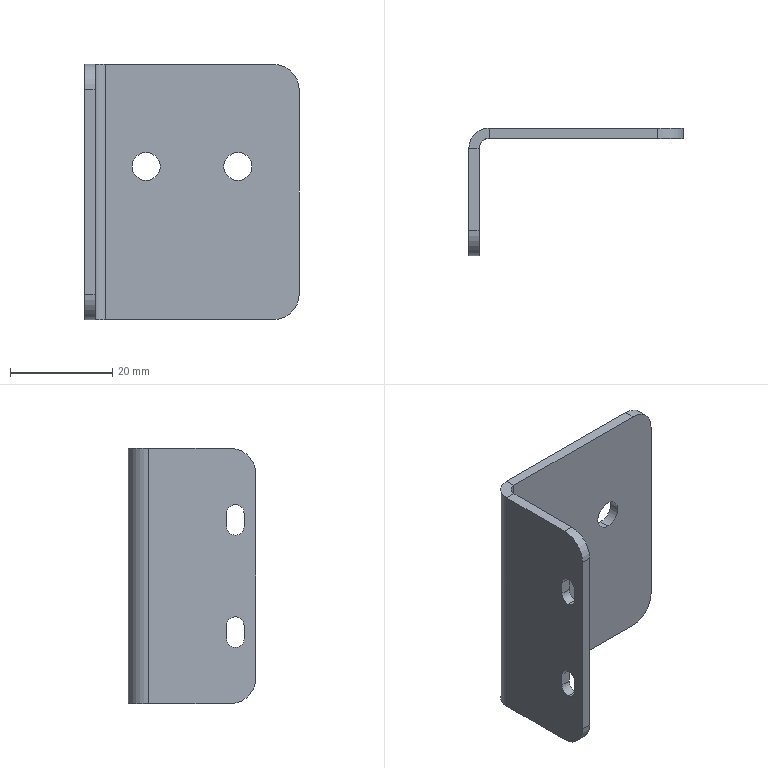Part | SolidWorks | features HoleWzd 3, EdgeFlange 2, Chamfer 1, Fillet 1, FlatPattern 1, MirrorPattern 1, SMBaseFlange 1, SheetMetal 1 | 1 solid | 32 faces | box 42 x 25 x 50 mm | volume 6162 mm3 | cylinder 16 | plane 16 | commonest cylinder face diameters 3.4 x6 5.5 x4 10 x4 4 x1 8 x1
STEP:
#1=CARTESIAN_POINT('',(28.,13.5,7.75));
#2=VERTEX_POINT('',#1);
#3=CARTESIAN_POINT('',(28.,13.5,2.25));
#4=VERTEX_POINT('',#3);
#5=CARTESIAN_POINT('',(28.,13.5,5.));
#6=DIRECTION('',(0.,-1.,0.));
#7=DIRECTION('',(0.,0.,-1.));
#8=AXIS2_PLACEMENT_3D('',#5,#6,#7);
#9=CIRCLE('',#8,2.75);
#10=EDGE_CURVE('',#2,#4,#9,.T.);
#11=ORIENTED_EDGE('',*,*,#10,.F.);
#12=CARTESIAN_POINT('',(28.,11.5,7.75));
#13=VERTEX_POINT('',#12);
#14=CARTESIAN_POINT('',(28.,11.5,7.75));
#15=DIRECTION('',(0.,-1.,0.));
#16=VECTOR('',#15,1000.);
#17=LINE('',#14,#16);
#18=EDGE_CURVE('',#2,#13,#17,.T.);
#19=ORIENTED_EDGE('',*,*,#18,.T.);
#20=CARTESIAN_POINT('',(28.,11.5,2.25));
#21=VERTEX_POINT('',#20);
#22=CARTESIAN_POINT('',(28.,11.5,5.));
#23=DIRECTION('',(0.,-1.,0.));
#24=DIRECTION('',(0.,0.,-1.));
#25=AXIS2_PLACEMENT_3D('',#22,#23,#24);
#26=CIRCLE('',#25,2.75);
#27=EDGE_CURVE('',#13,#21,#26,.T.);
#28=ORIENTED_EDGE('',*,*,#27,.T.);
#29=CARTESIAN_POINT('',(28.,11.5,2.25));
#30=DIRECTION('',(0.,-1.,0.));
#31=VECTOR('',#30,1000.);
#32=LINE('',#29,#31);
#33=EDGE_CURVE('',#4,#21,#32,.T.);
#34=ORIENTED_EDGE('',*,*,#33,.F.);
#35=EDGE_LOOP('',(#11,#19,#28,#34));
#36=FACE_OUTER_BOUND('',#35,.T.);
#37=CARTESIAN_POINT('',(28.,11.5,5.));
#38=DIRECTION('',(0.,-1.,0.));
#39=DIRECTION('',(0.,0.,-1.));
#40=AXIS2_PLACEMENT_3D('',#37,#38,#39);
#41=CYLINDRICAL_SURFACE('',#40,2.75);
#42=ADVANCED_FACE('',(#36),#41,.F.);
#43=CARTESIAN_POINT('',(10.,13.5,7.75));
#44=VERTEX_POINT('',#43);
#45=CARTESIAN_POINT('',(10.,13.5,2.25));
#46=VERTEX_POINT('',#45);
#47=CARTESIAN_POINT('',(10.,13.5,5.));
#48=DIRECTION('',(0.,-1.,0.));
#49=DIRECTION('',(0.,0.,-1.));
#50=AXIS2_PLACEMENT_3D('',#47,#48,#49);
#51=CIRCLE('',#50,2.75);
#52=EDGE_CURVE('',#44,#46,#51,.T.);
#53=ORIENTED_EDGE('',*,*,#52,.F.);
#54=CARTESIAN_POINT('',(10.,11.5,7.75));
#55=VERTEX_POINT('',#54);
#56=CARTESIAN_POINT('',(10.,11.5,7.75));
#57=DIRECTION('',(0.,-1.,0.));
#58=VECTOR('',#57,1000.);
#59=LINE('',#56,#58);
#60=EDGE_CURVE('',#44,#55,#59,.T.);
#61=ORIENTED_EDGE('',*,*,#60,.T.);
#62=CARTESIAN_POINT('',(10.,11.5,2.25));
#63=VERTEX_POINT('',#62);
#64=CARTESIAN_POINT('',(10.,11.5,5.));
#65=DIRECTION('',(0.,-1.,0.));
#66=DIRECTION('',(0.,0.,-1.));
#67=AXIS2_PLACEMENT_3D('',#64,#65,#66);
#68=CIRCLE('',#67,2.75);
#69=EDGE_CURVE('',#55,#63,#68,.T.);
#70=ORIENTED_EDGE('',*,*,#69,.T.);
#71=CARTESIAN_POINT('',(10.,11.5,2.25));
#72=DIRECTION('',(0.,-1.,0.));
#73=VECTOR('',#72,1000.);
#74=LINE('',#71,#73);
#75=EDGE_CURVE('',#46,#63,#74,.T.);
#76=ORIENTED_EDGE('',*,*,#75,.F.);
#77=EDGE_LOOP('',(#53,#61,#70,#76));
#78=FACE_OUTER_BOUND('',#77,.T.);
#79=CARTESIAN_POINT('',(10.,11.5,5.));
#80=DIRECTION('',(0.,-1.,0.));
#81=DIRECTION('',(0.,0.,-1.));
#82=AXIS2_PLACEMENT_3D('',#79,#80,#81);
#83=CYLINDRICAL_SURFACE('',#82,2.75);
#84=ADVANCED_FACE('',(#78),#83,.F.);
#85=CARTESIAN_POINT('',(-2.,-7.5,-14.));
#86=VERTEX_POINT('',#85);
#87=CARTESIAN_POINT('',(-2.,-5.8,-12.3));
#88=VERTEX_POINT('',#87);
#89=CARTESIAN_POINT('',(-2.,-7.5,-12.3));
#90=DIRECTION('',(1.,0.,0.));
#91=DIRECTION('',(0.,0.,-1.));
#92=AXIS2_PLACEMENT_3D('',#89,#90,#91);
#93=CIRCLE('',#92,1.7);
#94=EDGE_CURVE('',#86,#88,#93,.T.);
#95=ORIENTED_EDGE('',*,*,#94,.F.);
#96=CARTESIAN_POINT('',(0.,-7.5,-14.));
#97=VERTEX_POINT('',#96);
#98=CARTESIAN_POINT('',(0.,-7.5,-14.));
#99=DIRECTION('',(1.,0.,0.));
#100=VECTOR('',#99,1000.);
#101=LINE('',#98,#100);
#102=EDGE_CURVE('',#86,#97,#101,.T.);
#103=ORIENTED_EDGE('',*,*,#102,.T.);
#104=CARTESIAN_POINT('',(0.,-5.8,-12.3));
#105=VERTEX_POINT('',#104);
#106=CARTESIAN_POINT('',(0.,-7.5,-12.3));
#107=DIRECTION('',(1.,0.,0.));
#108=DIRECTION('',(0.,0.,-1.));
#109=AXIS2_PLACEMENT_3D('',#106,#107,#108);
#110=CIRCLE('',#109,1.7);
#111=EDGE_CURVE('',#97,#105,#110,.T.);
#112=ORIENTED_EDGE('',*,*,#111,.T.);
#113=CARTESIAN_POINT('',(-2.,-5.8,-12.3));
#114=DIRECTION('',(-1.,0.,0.));
#115=VECTOR('',#114,1000.);
#116=LINE('',#113,#115);
#117=EDGE_CURVE('',#105,#88,#116,.T.);
#118=ORIENTED_EDGE('',*,*,#117,.T.);
#119=EDGE_LOOP('',(#95,#103,#112,#118));
#120=FACE_OUTER_BOUND('',#119,.T.);
#121=CARTESIAN_POINT('',(0.,-7.5,-12.3));
#122=DIRECTION('',(1.,0.,0.));
#123=DIRECTION('',(0.,0.,-1.));
#124=AXIS2_PLACEMENT_3D('',#121,#122,#123);
#125=CYLINDRICAL_SURFACE('',#124,1.7);
#126=ADVANCED_FACE('',(#120),#125,.F.);
#127=CARTESIAN_POINT('',(-2.,-7.5,8.));
#128=VERTEX_POINT('',#127);
#129=CARTESIAN_POINT('',(-2.,-5.8,9.7));
#130=VERTEX_POINT('',#129);
#131=CARTESIAN_POINT('',(-2.,-7.5,9.7));
#132=DIRECTION('',(1.,0.,0.));
#133=DIRECTION('',(0.,0.,-1.));
#134=AXIS2_PLACEMENT_3D('',#131,#132,#133);
#135=CIRCLE('',#134,1.7);
#136=EDGE_CURVE('',#128,#130,#135,.T.);
#137=ORIENTED_EDGE('',*,*,#136,.F.);
#138=CARTESIAN_POINT('',(0.,-7.5,8.));
#139=VERTEX_POINT('',#138);
#140=CARTESIAN_POINT('',(0.,-7.5,8.));
#141=DIRECTION('',(1.,0.,0.));
#142=VECTOR('',#141,1000.);
#143=LINE('',#140,#142);
#144=EDGE_CURVE('',#128,#139,#143,.T.);
#145=ORIENTED_EDGE('',*,*,#144,.T.);
#146=CARTESIAN_POINT('',(0.,-5.8,9.7));
#147=VERTEX_POINT('',#146);
#148=CARTESIAN_POINT('',(0.,-7.5,9.7));
#149=DIRECTION('',(1.,0.,0.));
#150=DIRECTION('',(0.,0.,-1.));
#151=AXIS2_PLACEMENT_3D('',#148,#149,#150);
#152=CIRCLE('',#151,1.7);
#153=EDGE_CURVE('',#139,#147,#152,.T.);
#154=ORIENTED_EDGE('',*,*,#153,.T.);
#155=CARTESIAN_POINT('',(-2.,-5.8,9.7));
#156=DIRECTION('',(-1.,0.,0.));
#157=VECTOR('',#156,1000.);
#158=LINE('',#155,#157);
#159=EDGE_CURVE('',#147,#130,#158,.T.);
#160=ORIENTED_EDGE('',*,*,#159,.T.);
#161=EDGE_LOOP('',(#137,#145,#154,#160));
#162=FACE_OUTER_BOUND('',#161,.T.);
#163=CARTESIAN_POINT('',(0.,-7.5,9.7));
#164=DIRECTION('',(1.,0.,0.));
#165=DIRECTION('',(0.,0.,-1.));
#166=AXIS2_PLACEMENT_3D('',#163,#164,#165);
#167=CYLINDRICAL_SURFACE('',#166,1.7);
#168=ADVANCED_FACE('',(#162),#167,.F.);
#169=CARTESIAN_POINT('',(-2.,9.5,25.));
#170=VERTEX_POINT('',#169);
#171=CARTESIAN_POINT('',(-2.,-6.5,25.));
#172=VERTEX_POINT('',#171);
#173=CARTESIAN_POINT('',(-2.,11.5,25.));
#174=DIRECTION('',(0.,-1.,0.));
#175=VECTOR('',#174,1000.);
#176=LINE('',#173,#175);
#177=EDGE_CURVE('',#170,#172,#176,.T.);
#178=ORIENTED_EDGE('',*,*,#177,.T.);
#179=CARTESIAN_POINT('',(0.,-6.5,25.));
#180=VERTEX_POINT('',#179);
#181=CARTESIAN_POINT('',(-2.,-6.5,25.));
#182=DIRECTION('',(1.,0.,0.));
#183=VECTOR('',#182,1000.);
#184=LINE('',#181,#183);
#185=EDGE_CURVE('',#172,#180,#184,.T.);
#186=ORIENTED_EDGE('',*,*,#185,.T.);
#187=CARTESIAN_POINT('',(0.,9.5,25.));
#188=VERTEX_POINT('',#187);
#189=CARTESIAN_POINT('',(0.,11.5,25.));
#190=DIRECTION('',(0.,-1.,0.));
#191=VECTOR('',#190,1000.);
#192=LINE('',#189,#191);
#193=EDGE_CURVE('',#188,#180,#192,.T.);
#194=ORIENTED_EDGE('',*,*,#193,.F.);
#195=CARTESIAN_POINT('',(0.,9.5,25.));
#196=DIRECTION('',(-1.,0.,0.));
#197=VECTOR('',#196,1000.);
#198=LINE('',#195,#197);
#199=EDGE_CURVE('',#188,#170,#198,.T.);
#200=ORIENTED_EDGE('',*,*,#199,.T.);
#201=EDGE_LOOP('',(#178,#186,#194,#200));
#202=FACE_OUTER_BOUND('',#201,.T.);
#203=CARTESIAN_POINT('',(-2.,11.5,25.));
#204=DIRECTION('',(0.,0.,1.));
#205=DIRECTION('',(0.,-1.,0.));
#206=AXIS2_PLACEMENT_3D('',#203,#204,#205);
#207=PLANE('',#206);
#208=ADVANCED_FACE('',(#202),#207,.T.);
#209=CARTESIAN_POINT('',(-2.,-5.8,12.3));
#210=VERTEX_POINT('',#209);
#211=CARTESIAN_POINT('',(-2.,-9.2,12.3));
#212=VERTEX_POINT('',#211);
#213=CARTESIAN_POINT('',(-2.,-7.5,12.3));
#214=DIRECTION('',(1.,0.,0.));
#215=DIRECTION('',(0.,0.,-1.));
#216=AXIS2_PLACEMENT_3D('',#213,#214,#215);
#217=CIRCLE('',#216,1.7);
#218=EDGE_CURVE('',#210,#212,#217,.T.);
#219=ORIENTED_EDGE('',*,*,#218,.T.);
#220=CARTESIAN_POINT('',(-2.,-9.2,9.7));
#221=VERTEX_POINT('',#220);
#222=CARTESIAN_POINT('',(-2.,-9.2,12.3));
#223=DIRECTION('',(0.,0.,-1.));
#224=VECTOR('',#223,1000.);
#225=LINE('',#222,#224);
#226=EDGE_CURVE('',#212,#221,#225,.T.);
#227=ORIENTED_EDGE('',*,*,#226,.T.);
#228=CARTESIAN_POINT('',(-2.,-7.5,9.7));
#229=DIRECTION('',(1.,0.,0.));
#230=DIRECTION('',(0.,0.,-1.));
#231=AXIS2_PLACEMENT_3D('',#228,#229,#230);
#232=CIRCLE('',#231,1.7);
#233=EDGE_CURVE('',#221,#128,#232,.T.);
#234=ORIENTED_EDGE('',*,*,#233,.T.);
#235=ORIENTED_EDGE('',*,*,#136,.T.);
#236=CARTESIAN_POINT('',(-2.,-5.8,12.3));
#237=DIRECTION('',(0.,0.,-1.));
#238=VECTOR('',#237,1000.);
#239=LINE('',#236,#238);
#240=EDGE_CURVE('',#210,#130,#239,.T.);
#241=ORIENTED_EDGE('',*,*,#240,.F.);
#242=EDGE_LOOP('',(#219,#227,#234,#235,#241));
#243=FACE_BOUND('',#242,.T.);
#244=CARTESIAN_POINT('',(-2.,-5.8,-9.7));
#245=VERTEX_POINT('',#244);
#246=CARTESIAN_POINT('',(-2.,-5.8,-9.7));
#247=DIRECTION('',(0.,0.,-1.));
#248=VECTOR('',#247,1000.);
#249=LINE('',#246,#248);
#250=EDGE_CURVE('',#245,#88,#249,.T.);
#251=ORIENTED_EDGE('',*,*,#250,.F.);
#252=CARTESIAN_POINT('',(-2.,-9.2,-9.7));
#253=VERTEX_POINT('',#252);
#254=CARTESIAN_POINT('',(-2.,-7.5,-9.7));
#255=DIRECTION('',(1.,0.,0.));
#256=DIRECTION('',(0.,0.,-1.));
#257=AXIS2_PLACEMENT_3D('',#254,#255,#256);
#258=CIRCLE('',#257,1.7);
#259=EDGE_CURVE('',#245,#253,#258,.T.);
#260=ORIENTED_EDGE('',*,*,#259,.T.);
#261=CARTESIAN_POINT('',(-2.,-9.2,-12.3));
#262=VERTEX_POINT('',#261);
#263=CARTESIAN_POINT('',(-2.,-9.2,-9.7));
#264=DIRECTION('',(0.,0.,-1.));
#265=VECTOR('',#264,1000.);
#266=LINE('',#263,#265);
#267=EDGE_CURVE('',#253,#262,#266,.T.);
#268=ORIENTED_EDGE('',*,*,#267,.T.);
#269=CARTESIAN_POINT('',(-2.,-7.5,-12.3));
#270=DIRECTION('',(1.,0.,0.));
#271=DIRECTION('',(0.,0.,-1.));
#272=AXIS2_PLACEMENT_3D('',#269,#270,#271);
#273=CIRCLE('',#272,1.7);
#274=EDGE_CURVE('',#262,#86,#273,.T.);
#275=ORIENTED_EDGE('',*,*,#274,.T.);
#276=ORIENTED_EDGE('',*,*,#94,.T.);
#277=EDGE_LOOP('',(#251,#260,#268,#275,#276));
#278=FACE_BOUND('',#277,.T.);
#279=CARTESIAN_POINT('',(-2.,-11.5,20.));
#280=VERTEX_POINT('',#279);
#281=CARTESIAN_POINT('',(-2.,-11.5,-20.));
#282=VERTEX_POINT('',#281);
#283=CARTESIAN_POINT('',(-2.,-11.5,25.));
#284=DIRECTION('',(0.,0.,-1.));
#285=VECTOR('',#284,1000.);
#286=LINE('',#283,#285);
#287=EDGE_CURVE('',#280,#282,#286,.T.);
#288=ORIENTED_EDGE('',*,*,#287,.F.);
#289=CARTESIAN_POINT('',(-2.,-6.5,20.));
#290=DIRECTION('',(-1.,0.,0.));
#291=DIRECTION('',(0.,0.,-1.));
#292=AXIS2_PLACEMENT_3D('',#289,#290,#291);
#293=CIRCLE('',#292,5.);
#294=EDGE_CURVE('',#280,#172,#293,.T.);
#295=ORIENTED_EDGE('',*,*,#294,.T.);
#296=ORIENTED_EDGE('',*,*,#177,.F.);
#297=CARTESIAN_POINT('',(-2.,9.5,-25.));
#298=VERTEX_POINT('',#297);
#299=CARTESIAN_POINT('',(-2.,9.5,25.));
#300=DIRECTION('',(0.,0.,-1.));
#301=VECTOR('',#300,1000.);
#302=LINE('',#299,#301);
#303=EDGE_CURVE('',#170,#298,#302,.T.);
#304=ORIENTED_EDGE('',*,*,#303,.T.);
#305=CARTESIAN_POINT('',(-2.,-6.5,-25.));
#306=VERTEX_POINT('',#305);
#307=CARTESIAN_POINT('',(-2.,11.5,-25.));
#308=DIRECTION('',(0.,1.,0.));
#309=VECTOR('',#308,1000.);
#310=LINE('',#307,#309);
#311=EDGE_CURVE('',#306,#298,#310,.T.);
#312=ORIENTED_EDGE('',*,*,#311,.F.);
#313=CARTESIAN_POINT('',(-2.,-6.5,-20.));
#314=DIRECTION('',(-1.,0.,0.));
#315=DIRECTION('',(0.,0.,-1.));
#316=AXIS2_PLACEMENT_3D('',#313,#314,#315);
#317=CIRCLE('',#316,5.);
#318=EDGE_CURVE('',#306,#282,#317,.T.);
#319=ORIENTED_EDGE('',*,*,#318,.T.);
#320=EDGE_LOOP('',(#288,#295,#296,#304,#312,#319));
#321=FACE_OUTER_BOUND('',#320,.T.);
#322=CARTESIAN_POINT('',(-2.,0.,0.));
#323=DIRECTION('',(1.,0.,0.));
#324=DIRECTION('',(0.,0.,-1.));
#325=AXIS2_PLACEMENT_3D('',#322,#323,#324);
#326=PLANE('',#325);
#327=ADVANCED_FACE('',(#243,#278,#321),#326,.F.);
#328=CARTESIAN_POINT('',(0.,-9.2,-12.3));
#329=VERTEX_POINT('',#328);
#330=CARTESIAN_POINT('',(0.,-7.5,-12.3));
#331=DIRECTION('',(1.,0.,0.));
#332=DIRECTION('',(0.,0.,-1.));
#333=AXIS2_PLACEMENT_3D('',#330,#331,#332);
#334=CIRCLE('',#333,1.7);
#335=EDGE_CURVE('',#329,#97,#334,.T.);
#336=ORIENTED_EDGE('',*,*,#335,.F.);
#337=CARTESIAN_POINT('',(0.,-9.2,-9.7));
#338=VERTEX_POINT('',#337);
#339=CARTESIAN_POINT('',(0.,-9.2,-9.7));
#340=DIRECTION('',(0.,0.,-1.));
#341=VECTOR('',#340,1000.);
#342=LINE('',#339,#341);
#343=EDGE_CURVE('',#338,#329,#342,.T.);
#344=ORIENTED_EDGE('',*,*,#343,.F.);
#345=CARTESIAN_POINT('',(0.,-5.8,-9.7));
#346=VERTEX_POINT('',#345);
#347=CARTESIAN_POINT('',(0.,-7.5,-9.7));
#348=DIRECTION('',(1.,0.,0.));
#349=DIRECTION('',(0.,0.,-1.));
#350=AXIS2_PLACEMENT_3D('',#347,#348,#349);
#351=CIRCLE('',#350,1.7);
#352=EDGE_CURVE('',#346,#338,#351,.T.);
#353=ORIENTED_EDGE('',*,*,#352,.F.);
#354=CARTESIAN_POINT('',(0.,-5.8,-9.7));
#355=DIRECTION('',(0.,0.,-1.));
#356=VECTOR('',#355,1000.);
#357=LINE('',#354,#356);
#358=EDGE_CURVE('',#346,#105,#357,.T.);
#359=ORIENTED_EDGE('',*,*,#358,.T.);
#360=ORIENTED_EDGE('',*,*,#111,.F.);
#361=EDGE_LOOP('',(#336,#344,#353,#359,#360));
#362=FACE_BOUND('',#361,.T.);
#363=CARTESIAN_POINT('',(0.,-9.2,12.3));
#364=VERTEX_POINT('',#363);
#365=CARTESIAN_POINT('',(0.,-9.2,9.7));
#366=VERTEX_POINT('',#365);
#367=CARTESIAN_POINT('',(0.,-9.2,12.3));
#368=DIRECTION('',(0.,0.,-1.));
#369=VECTOR('',#368,1000.);
#370=LINE('',#367,#369);
#371=EDGE_CURVE('',#364,#366,#370,.T.);
#372=ORIENTED_EDGE('',*,*,#371,.F.);
#373=CARTESIAN_POINT('',(0.,-5.8,12.3));
#374=VERTEX_POINT('',#373);
#375=CARTESIAN_POINT('',(0.,-7.5,12.3));
#376=DIRECTION('',(1.,0.,0.));
#377=DIRECTION('',(0.,0.,-1.));
#378=AXIS2_PLACEMENT_3D('',#375,#376,#377);
#379=CIRCLE('',#378,1.7);
#380=EDGE_CURVE('',#374,#364,#379,.T.);
#381=ORIENTED_EDGE('',*,*,#380,.F.);
#382=CARTESIAN_POINT('',(0.,-5.8,12.3));
#383=DIRECTION('',(0.,0.,-1.));
#384=VECTOR('',#383,1000.);
#385=LINE('',#382,#384);
#386=EDGE_CURVE('',#374,#147,#385,.T.);
#387=ORIENTED_EDGE('',*,*,#386,.T.);
#388=ORIENTED_EDGE('',*,*,#153,.F.);
#389=CARTESIAN_POINT('',(0.,-7.5,9.7));
#390=DIRECTION('',(1.,0.,0.));
#391=DIRECTION('',(0.,0.,-1.));
#392=AXIS2_PLACEMENT_3D('',#389,#390,#391);
#393=CIRCLE('',#392,1.7);
#394=EDGE_CURVE('',#366,#139,#393,.T.);
#395=ORIENTED_EDGE('',*,*,#394,.F.);
#396=EDGE_LOOP('',(#372,#381,#387,#388,#395));
#397=FACE_BOUND('',#396,.T.);
#398=ORIENTED_EDGE('',*,*,#193,.T.);
#399=CARTESIAN_POINT('',(0.,-11.5,20.));
#400=VERTEX_POINT('',#399);
#401=CARTESIAN_POINT('',(0.,-6.5,20.));
#402=DIRECTION('',(1.,0.,0.));
#403=DIRECTION('',(0.,0.,-1.));
#404=AXIS2_PLACEMENT_3D('',#401,#402,#403);
#405=CIRCLE('',#404,5.);
#406=EDGE_CURVE('',#180,#400,#405,.T.);
#407=ORIENTED_EDGE('',*,*,#406,.T.);
#408=CARTESIAN_POINT('',(0.,-11.5,-20.));
#409=VERTEX_POINT('',#408);
#410=CARTESIAN_POINT('',(0.,-11.5,25.));
#411=DIRECTION('',(0.,0.,-1.));
#412=VECTOR('',#411,1000.);
#413=LINE('',#410,#412);
#414=EDGE_CURVE('',#400,#409,#413,.T.);
#415=ORIENTED_EDGE('',*,*,#414,.T.);
#416=CARTESIAN_POINT('',(0.,-6.5,-25.));
#417=VERTEX_POINT('',#416);
#418=CARTESIAN_POINT('',(0.,-6.5,-20.));
#419=DIRECTION('',(1.,0.,0.));
#420=DIRECTION('',(0.,0.,-1.));
#421=AXIS2_PLACEMENT_3D('',#418,#419,#420);
#422=CIRCLE('',#421,5.);
#423=EDGE_CURVE('',#409,#417,#422,.T.);
#424=ORIENTED_EDGE('',*,*,#423,.T.);
#425=CARTESIAN_POINT('',(0.,9.5,-25.));
#426=VERTEX_POINT('',#425);
#427=CARTESIAN_POINT('',(0.,11.5,-25.));
#428=DIRECTION('',(0.,1.,0.));
#429=VECTOR('',#428,1000.);
#430=LINE('',#427,#429);
#431=EDGE_CURVE('',#417,#426,#430,.T.);
#432=ORIENTED_EDGE('',*,*,#431,.T.);
#433=CARTESIAN_POINT('',(0.,9.5,25.));
#434=DIRECTION('',(0.,0.,-1.));
#435=VECTOR('',#434,1000.);
#436=LINE('',#433,#435);
#437=EDGE_CURVE('',#188,#426,#436,.T.);
#438=ORIENTED_EDGE('',*,*,#437,.F.);
#439=EDGE_LOOP('',(#398,#407,#415,#424,#432,#438));
#440=FACE_OUTER_BOUND('',#439,.T.);
#441=CARTESIAN_POINT('',(0.,0.,0.));
#442=DIRECTION('',(1.,0.,0.));
#443=DIRECTION('',(0.,0.,-1.));
#444=AXIS2_PLACEMENT_3D('',#441,#442,#443);
#445=PLANE('',#444);
#446=ADVANCED_FACE('',(#362,#397,#440),#445,.T.);
#447=ORIENTED_EDGE('',*,*,#431,.F.);
#448=CARTESIAN_POINT('',(-2.,-6.5,-25.));
#449=DIRECTION('',(-1.,0.,0.));
#450=VECTOR('',#449,1000.);
#451=LINE('',#448,#450);
#452=EDGE_CURVE('',#417,#306,#451,.T.);
#453=ORIENTED_EDGE('',*,*,#452,.T.);
#454=ORIENTED_EDGE('',*,*,#311,.T.);
#455=CARTESIAN_POINT('',(0.,9.5,-25.));
#456=DIRECTION('',(-1.,0.,0.));
#457=VECTOR('',#456,1000.);
#458=LINE('',#455,#457);
#459=EDGE_CURVE('',#426,#298,#458,.T.);
#460=ORIENTED_EDGE('',*,*,#459,.F.);
#461=EDGE_LOOP('',(#447,#453,#454,#460));
#462=FACE_OUTER_BOUND('',#461,.T.);
#463=CARTESIAN_POINT('',(-2.,11.5,-25.));
#464=DIRECTION('',(0.,0.,-1.));
#465=DIRECTION('',(0.,1.,0.));
#466=AXIS2_PLACEMENT_3D('',#463,#464,#465);
#467=PLANE('',#466);
#468=ADVANCED_FACE('',(#462),#467,.T.);
#469=ORIENTED_EDGE('',*,*,#414,.F.);
#470=CARTESIAN_POINT('',(-2.,-11.5,20.));
#471=DIRECTION('',(-1.,0.,0.));
#472=VECTOR('',#471,1000.);
#473=LINE('',#470,#472);
#474=EDGE_CURVE('',#400,#280,#473,.T.);
#475=ORIENTED_EDGE('',*,*,#474,.T.);
#476=ORIENTED_EDGE('',*,*,#287,.T.);
#477=CARTESIAN_POINT('',(-2.,-11.5,-20.));
#478=DIRECTION('',(1.,0.,0.));
#479=VECTOR('',#478,1000.);
#480=LINE('',#477,#479);
#481=EDGE_CURVE('',#282,#409,#480,.T.);
#482=ORIENTED_EDGE('',*,*,#481,.T.);
#483=EDGE_LOOP('',(#469,#475,#476,#482));
#484=FACE_OUTER_BOUND('',#483,.T.);
#485=CARTESIAN_POINT('',(-2.,-11.5,25.));
#486=DIRECTION('',(0.,-1.,0.));
#487=DIRECTION('',(0.,0.,-1.));
#488=AXIS2_PLACEMENT_3D('',#485,#486,#487);
#489=PLANE('',#488);
#490=ADVANCED_FACE('',(#484),#489,.T.);
#491=ORIENTED_EDGE('',*,*,#144,.F.);
#492=ORIENTED_EDGE('',*,*,#233,.F.);
#493=CARTESIAN_POINT('',(0.,-9.2,9.7));
#494=DIRECTION('',(-1.,0.,0.));
#495=VECTOR('',#494,1000.);
#496=LINE('',#493,#495);
#497=EDGE_CURVE('',#366,#221,#496,.T.);
#498=ORIENTED_EDGE('',*,*,#497,.F.);
#499=ORIENTED_EDGE('',*,*,#394,.T.);
#500=EDGE_LOOP('',(#491,#492,#498,#499));
#501=FACE_OUTER_BOUND('',#500,.T.);
#502=CARTESIAN_POINT('',(0.,-7.5,9.7));
#503=DIRECTION('',(1.,0.,0.));
#504=DIRECTION('',(0.,0.,-1.));
#505=AXIS2_PLACEMENT_3D('',#502,#503,#504);
#506=CYLINDRICAL_SURFACE('',#505,1.7);
#507=ADVANCED_FACE('',(#501),#506,.F.);
#508=ORIENTED_EDGE('',*,*,#218,.F.);
#509=CARTESIAN_POINT('',(-2.,-5.8,12.3));
#510=DIRECTION('',(-1.,0.,0.));
#511=VECTOR('',#510,1000.);
#512=LINE('',#509,#511);
#513=EDGE_CURVE('',#374,#210,#512,.T.);
#514=ORIENTED_EDGE('',*,*,#513,.F.);
#515=ORIENTED_EDGE('',*,*,#380,.T.);
#516=CARTESIAN_POINT('',(0.,-9.2,12.3));
#517=DIRECTION('',(1.,0.,0.));
#518=VECTOR('',#517,1000.);
#519=LINE('',#516,#518);
#520=EDGE_CURVE('',#212,#364,#519,.T.);
#521=ORIENTED_EDGE('',*,*,#520,.F.);
#522=EDGE_LOOP('',(#508,#514,#515,#521));
#523=FACE_OUTER_BOUND('',#522,.T.);
#524=CARTESIAN_POINT('',(0.,-7.5,12.3));
#525=DIRECTION('',(1.,0.,0.));
#526=DIRECTION('',(0.,0.,-1.));
#527=AXIS2_PLACEMENT_3D('',#524,#525,#526);
#528=CYLINDRICAL_SURFACE('',#527,1.7);
#529=ADVANCED_FACE('',(#523),#528,.F.);
#530=ORIENTED_EDGE('',*,*,#159,.F.);
#531=ORIENTED_EDGE('',*,*,#386,.F.);
#532=ORIENTED_EDGE('',*,*,#513,.T.);
#533=ORIENTED_EDGE('',*,*,#240,.T.);
#534=EDGE_LOOP('',(#530,#531,#532,#533));
#535=FACE_OUTER_BOUND('',#534,.T.);
#536=CARTESIAN_POINT('',(-2.,-5.8,12.3));
#537=DIRECTION('',(0.,-1.,0.));
#538=DIRECTION('',(1.,0.,0.));
#539=AXIS2_PLACEMENT_3D('',#536,#537,#538);
#540=PLANE('',#539);
#541=ADVANCED_FACE('',(#535),#540,.T.);
#542=ORIENTED_EDGE('',*,*,#497,.T.);
#543=ORIENTED_EDGE('',*,*,#226,.F.);
#544=ORIENTED_EDGE('',*,*,#520,.T.);
#545=ORIENTED_EDGE('',*,*,#371,.T.);
#546=EDGE_LOOP('',(#542,#543,#544,#545));
#547=FACE_OUTER_BOUND('',#546,.T.);
#548=CARTESIAN_POINT('',(0.,-9.2,12.3));
#549=DIRECTION('',(0.,-1.,0.));
#550=DIRECTION('',(0.,0.,-1.));
#551=AXIS2_PLACEMENT_3D('',#548,#549,#550);
#552=PLANE('',#551);
#553=ADVANCED_FACE('',(#547),#552,.F.);
#554=ORIENTED_EDGE('',*,*,#102,.F.);
#555=ORIENTED_EDGE('',*,*,#274,.F.);
#556=CARTESIAN_POINT('',(0.,-9.2,-12.3));
#557=DIRECTION('',(-1.,0.,0.));
#558=VECTOR('',#557,1000.);
#559=LINE('',#556,#558);
#560=EDGE_CURVE('',#329,#262,#559,.T.);
#561=ORIENTED_EDGE('',*,*,#560,.F.);
#562=ORIENTED_EDGE('',*,*,#335,.T.);
#563=EDGE_LOOP('',(#554,#555,#561,#562));
#564=FACE_OUTER_BOUND('',#563,.T.);
#565=CARTESIAN_POINT('',(0.,-7.5,-12.3));
#566=DIRECTION('',(1.,0.,0.));
#567=DIRECTION('',(0.,0.,-1.));
#568=AXIS2_PLACEMENT_3D('',#565,#566,#567);
#569=CYLINDRICAL_SURFACE('',#568,1.7);
#570=ADVANCED_FACE('',(#564),#569,.F.);
#571=ORIENTED_EDGE('',*,*,#259,.F.);
#572=CARTESIAN_POINT('',(-2.,-5.8,-9.7));
#573=DIRECTION('',(-1.,0.,0.));
#574=VECTOR('',#573,1000.);
#575=LINE('',#572,#574);
#576=EDGE_CURVE('',#346,#245,#575,.T.);
#577=ORIENTED_EDGE('',*,*,#576,.F.);
#578=ORIENTED_EDGE('',*,*,#352,.T.);
#579=CARTESIAN_POINT('',(0.,-9.2,-9.7));
#580=DIRECTION('',(1.,0.,0.));
#581=VECTOR('',#580,1000.);
#582=LINE('',#579,#581);
#583=EDGE_CURVE('',#253,#338,#582,.T.);
#584=ORIENTED_EDGE('',*,*,#583,.F.);
#585=EDGE_LOOP('',(#571,#577,#578,#584));
#586=FACE_OUTER_BOUND('',#585,.T.);
#587=CARTESIAN_POINT('',(0.,-7.5,-9.7));
#588=DIRECTION('',(1.,0.,0.));
#589=DIRECTION('',(0.,0.,-1.));
#590=AXIS2_PLACEMENT_3D('',#587,#588,#589);
#591=CYLINDRICAL_SURFACE('',#590,1.7);
#592=ADVANCED_FACE('',(#586),#591,.F.);
#593=ORIENTED_EDGE('',*,*,#117,.F.);
#594=ORIENTED_EDGE('',*,*,#358,.F.);
#595=ORIENTED_EDGE('',*,*,#576,.T.);
#596=ORIENTED_EDGE('',*,*,#250,.T.);
#597=EDGE_LOOP('',(#593,#594,#595,#596));
#598=FACE_OUTER_BOUND('',#597,.T.);
#599=CARTESIAN_POINT('',(-2.,-5.8,-9.7));
#600=DIRECTION('',(0.,-1.,0.));
#601=DIRECTION('',(1.,0.,0.));
#602=AXIS2_PLACEMENT_3D('',#599,#600,#601);
#603=PLANE('',#602);
#604=ADVANCED_FACE('',(#598),#603,.T.);
#605=ORIENTED_EDGE('',*,*,#560,.T.);
#606=ORIENTED_EDGE('',*,*,#267,.F.);
#607=ORIENTED_EDGE('',*,*,#583,.T.);
#608=ORIENTED_EDGE('',*,*,#343,.T.);
#609=EDGE_LOOP('',(#605,#606,#607,#608));
#610=FACE_OUTER_BOUND('',#609,.T.);
#611=CARTESIAN_POINT('',(0.,-9.2,-9.7));
#612=DIRECTION('',(0.,-1.,0.));
#613=DIRECTION('',(0.,0.,-1.));
#614=AXIS2_PLACEMENT_3D('',#611,#612,#613);
#615=PLANE('',#614);
#616=ADVANCED_FACE('',(#610),#615,.F.);
#617=CARTESIAN_POINT('',(2.,11.5,-25.));
#618=VERTEX_POINT('',#617);
#619=CARTESIAN_POINT('',(2.,13.5,-25.));
#620=VERTEX_POINT('',#619);
#621=CARTESIAN_POINT('',(2.,11.5,-25.));
#622=DIRECTION('',(0.,1.,0.));
#623=VECTOR('',#622,1000.);
#624=LINE('',#621,#623);
#625=EDGE_CURVE('',#618,#620,#624,.T.);
#626=ORIENTED_EDGE('',*,*,#625,.F.);
#627=CARTESIAN_POINT('',(2.,9.5,-25.));
#628=DIRECTION('',(0.,0.,-1.));
#629=DIRECTION('',(1.,0.,0.));
#630=AXIS2_PLACEMENT_3D('',#627,#628,#629);
#631=CIRCLE('',#630,2.);
#632=EDGE_CURVE('',#426,#618,#631,.T.);
#633=ORIENTED_EDGE('',*,*,#632,.F.);
#634=ORIENTED_EDGE('',*,*,#459,.T.);
#635=CARTESIAN_POINT('',(2.,9.5,-25.));
#636=DIRECTION('',(0.,0.,-1.));
#637=DIRECTION('',(1.,0.,0.));
#638=AXIS2_PLACEMENT_3D('',#635,#636,#637);
#639=CIRCLE('',#638,4.);
#640=EDGE_CURVE('',#298,#620,#639,.T.);
#641=ORIENTED_EDGE('',*,*,#640,.T.);
#642=EDGE_LOOP('',(#626,#633,#634,#641));
#643=FACE_OUTER_BOUND('',#642,.T.);
#644=CARTESIAN_POINT('',(2.,9.5,-25.));
#645=DIRECTION('',(0.,0.,-1.));
#646=DIRECTION('',(-1.,0.,0.));
#647=AXIS2_PLACEMENT_3D('',#644,#645,#646);
#648=PLANE('',#647);
#649=ADVANCED_FACE('',(#643),#648,.T.);
#650=CARTESIAN_POINT('',(2.,11.5,25.));
#651=VERTEX_POINT('',#650);
#652=CARTESIAN_POINT('',(2.,9.5,25.));
#653=DIRECTION('',(0.,0.,1.));
#654=DIRECTION('',(1.,0.,0.));
#655=AXIS2_PLACEMENT_3D('',#652,#653,#654);
#656=CIRCLE('',#655,2.);
#657=EDGE_CURVE('',#651,#188,#656,.T.);
#658=ORIENTED_EDGE('',*,*,#657,.F.);
#659=CARTESIAN_POINT('',(2.,13.5,25.));
#660=VERTEX_POINT('',#659);
#661=CARTESIAN_POINT('',(2.,11.5,25.));
#662=DIRECTION('',(0.,1.,0.));
#663=VECTOR('',#662,1000.);
#664=LINE('',#661,#663);
#665=EDGE_CURVE('',#651,#660,#664,.T.);
#666=ORIENTED_EDGE('',*,*,#665,.T.);
#667=CARTESIAN_POINT('',(2.,9.5,25.));
#668=DIRECTION('',(0.,0.,1.));
#669=DIRECTION('',(1.,0.,0.));
#670=AXIS2_PLACEMENT_3D('',#667,#668,#669);
#671=CIRCLE('',#670,4.);
#672=EDGE_CURVE('',#660,#170,#671,.T.);
#673=ORIENTED_EDGE('',*,*,#672,.T.);
#674=ORIENTED_EDGE('',*,*,#199,.F.);
#675=EDGE_LOOP('',(#658,#666,#673,#674));
#676=FACE_OUTER_BOUND('',#675,.T.);
#677=CARTESIAN_POINT('',(2.,9.5,25.));
#678=DIRECTION('',(0.,0.,-1.));
#679=DIRECTION('',(-1.,0.,0.));
#680=AXIS2_PLACEMENT_3D('',#677,#678,#679);
#681=PLANE('',#680);
#682=ADVANCED_FACE('',(#676),#681,.F.);
#683=ORIENTED_EDGE('',*,*,#303,.F.);
#684=ORIENTED_EDGE('',*,*,#672,.F.);
#685=CARTESIAN_POINT('',(2.,13.5,0.));
#686=DIRECTION('',(0.,0.,-1.));
#687=VECTOR('',#686,1000.);
#688=LINE('',#685,#687);
#689=EDGE_CURVE('',#660,#620,#688,.T.);
#690=ORIENTED_EDGE('',*,*,#689,.T.);
#691=ORIENTED_EDGE('',*,*,#640,.F.);
#692=EDGE_LOOP('',(#683,#684,#690,#691));
#693=FACE_OUTER_BOUND('',#692,.T.);
#694=CARTESIAN_POINT('',(2.,9.5,25.));
#695=DIRECTION('',(0.,0.,1.));
#696=DIRECTION('',(0.,1.,0.));
#697=AXIS2_PLACEMENT_3D('',#694,#695,#696);
#698=CYLINDRICAL_SURFACE('',#697,4.);
#699=ADVANCED_FACE('',(#693),#698,.T.);
#700=ORIENTED_EDGE('',*,*,#437,.T.);
#701=ORIENTED_EDGE('',*,*,#632,.T.);
#702=CARTESIAN_POINT('',(2.,11.5,-25.));
#703=DIRECTION('',(0.,0.,1.));
#704=VECTOR('',#703,1000.);
#705=LINE('',#702,#704);
#706=EDGE_CURVE('',#618,#651,#705,.T.);
#707=ORIENTED_EDGE('',*,*,#706,.T.);
#708=ORIENTED_EDGE('',*,*,#657,.T.);
#709=EDGE_LOOP('',(#700,#701,#707,#708));
#710=FACE_OUTER_BOUND('',#709,.T.);
#711=CARTESIAN_POINT('',(2.,9.5,25.));
#712=DIRECTION('',(0.,0.,1.));
#713=DIRECTION('',(0.,1.,0.));
#714=AXIS2_PLACEMENT_3D('',#711,#712,#713);
#715=CYLINDRICAL_SURFACE('',#714,2.);
#716=ADVANCED_FACE('',(#710),#715,.F.);
#717=CARTESIAN_POINT('',(35.,13.5,-25.));
#718=VERTEX_POINT('',#717);
#719=CARTESIAN_POINT('',(0.,13.5,-25.));
#720=DIRECTION('',(-1.,0.,0.));
#721=VECTOR('',#720,1000.);
#722=LINE('',#719,#721);
#723=EDGE_CURVE('',#718,#620,#722,.T.);
#724=ORIENTED_EDGE('',*,*,#723,.F.);
#725=CARTESIAN_POINT('',(35.,11.5,-25.));
#726=VERTEX_POINT('',#725);
#727=CARTESIAN_POINT('',(35.,13.5,-25.));
#728=DIRECTION('',(0.,-1.,0.));
#729=VECTOR('',#728,1000.);
#730=LINE('',#727,#729);
#731=EDGE_CURVE('',#718,#726,#730,.T.);
#732=ORIENTED_EDGE('',*,*,#731,.T.);
#733=CARTESIAN_POINT('',(0.,11.5,-25.));
#734=DIRECTION('',(-1.,0.,0.));
#735=VECTOR('',#734,1000.);
#736=LINE('',#733,#735);
#737=EDGE_CURVE('',#726,#618,#736,.T.);
#738=ORIENTED_EDGE('',*,*,#737,.T.);
#739=ORIENTED_EDGE('',*,*,#625,.T.);
#740=EDGE_LOOP('',(#724,#732,#738,#739));
#741=FACE_OUTER_BOUND('',#740,.T.);
#742=CARTESIAN_POINT('',(0.,13.5,-25.));
#743=DIRECTION('',(0.,0.,1.));
#744=DIRECTION('',(1.,0.,0.));
#745=AXIS2_PLACEMENT_3D('',#742,#743,#744);
#746=PLANE('',#745);
#747=ADVANCED_FACE('',(#741),#746,.F.);
#748=CARTESIAN_POINT('',(35.,11.5,25.));
#749=VERTEX_POINT('',#748);
#750=CARTESIAN_POINT('',(40.,11.5,25.));
#751=DIRECTION('',(1.,0.,0.));
#752=VECTOR('',#751,1000.);
#753=LINE('',#750,#752);
#754=EDGE_CURVE('',#651,#749,#753,.T.);
#755=ORIENTED_EDGE('',*,*,#754,.T.);
#756=CARTESIAN_POINT('',(35.,13.5,25.));
#757=VERTEX_POINT('',#756);
#758=CARTESIAN_POINT('',(35.,13.5,25.));
#759=DIRECTION('',(0.,1.,0.));
#760=VECTOR('',#759,1000.);
#761=LINE('',#758,#760);
#762=EDGE_CURVE('',#749,#757,#761,.T.);
#763=ORIENTED_EDGE('',*,*,#762,.T.);
#764=CARTESIAN_POINT('',(40.,13.5,25.));
#765=DIRECTION('',(1.,0.,0.));
#766=VECTOR('',#765,1000.);
#767=LINE('',#764,#766);
#768=EDGE_CURVE('',#660,#757,#767,.T.);
#769=ORIENTED_EDGE('',*,*,#768,.F.);
#770=ORIENTED_EDGE('',*,*,#665,.F.);
#771=EDGE_LOOP('',(#755,#763,#769,#770));
#772=FACE_OUTER_BOUND('',#771,.T.);
#773=CARTESIAN_POINT('',(40.,13.5,25.));
#774=DIRECTION('',(0.,0.,-1.));
#775=DIRECTION('',(-1.,0.,0.));
#776=AXIS2_PLACEMENT_3D('',#773,#774,#775);
#777=PLANE('',#776);
#778=ADVANCED_FACE('',(#772),#777,.F.);
#779=CARTESIAN_POINT('',(28.,13.5,5.));
#780=DIRECTION('',(0.,-1.,0.));
#781=DIRECTION('',(0.,0.,-1.));
#782=AXIS2_PLACEMENT_3D('',#779,#780,#781);
#783=CIRCLE('',#782,2.75);
#784=EDGE_CURVE('',#4,#2,#783,.T.);
#785=ORIENTED_EDGE('',*,*,#784,.T.);
#786=ORIENTED_EDGE('',*,*,#10,.T.);
#787=EDGE_LOOP('',(#785,#786));
#788=FACE_BOUND('',#787,.T.);
#789=CARTESIAN_POINT('',(10.,13.5,5.));
#790=DIRECTION('',(0.,-1.,0.));
#791=DIRECTION('',(0.,0.,-1.));
#792=AXIS2_PLACEMENT_3D('',#789,#790,#791);
#793=CIRCLE('',#792,2.75);
#794=EDGE_CURVE('',#46,#44,#793,.T.);
#795=ORIENTED_EDGE('',*,*,#794,.T.);
#796=ORIENTED_EDGE('',*,*,#52,.T.);
#797=EDGE_LOOP('',(#795,#796));
#798=FACE_BOUND('',#797,.T.);
#799=ORIENTED_EDGE('',*,*,#768,.T.);
#800=CARTESIAN_POINT('',(40.,13.5,20.));
#801=VERTEX_POINT('',#800);
#802=CARTESIAN_POINT('',(35.,13.5,20.));
#803=DIRECTION('',(0.,1.,0.));
#804=DIRECTION('',(1.,0.,0.));
#805=AXIS2_PLACEMENT_3D('',#802,#803,#804);
#806=CIRCLE('',#805,5.);
#807=EDGE_CURVE('',#757,#801,#806,.T.);
#808=ORIENTED_EDGE('',*,*,#807,.T.);
#809=CARTESIAN_POINT('',(40.,13.5,-20.));
#810=VERTEX_POINT('',#809);
#811=CARTESIAN_POINT('',(40.,13.5,-25.));
#812=DIRECTION('',(0.,0.,-1.));
#813=VECTOR('',#812,1000.);
#814=LINE('',#811,#813);
#815=EDGE_CURVE('',#801,#810,#814,.T.);
#816=ORIENTED_EDGE('',*,*,#815,.T.);
#817=CARTESIAN_POINT('',(35.,13.5,-20.));
#818=DIRECTION('',(0.,1.,0.));
#819=DIRECTION('',(1.,0.,0.));
#820=AXIS2_PLACEMENT_3D('',#817,#818,#819);
#821=CIRCLE('',#820,5.);
#822=EDGE_CURVE('',#810,#718,#821,.T.);
#823=ORIENTED_EDGE('',*,*,#822,.T.);
#824=ORIENTED_EDGE('',*,*,#723,.T.);
#825=ORIENTED_EDGE('',*,*,#689,.F.);
#826=EDGE_LOOP('',(#799,#808,#816,#823,#824,#825));
#827=FACE_OUTER_BOUND('',#826,.T.);
#828=CARTESIAN_POINT('',(0.,13.5,0.));
#829=DIRECTION('',(0.,-1.,0.));
#830=DIRECTION('',(1.,0.,0.));
#831=AXIS2_PLACEMENT_3D('',#828,#829,#830);
#832=PLANE('',#831);
#833=ADVANCED_FACE('',(#788,#798,#827),#832,.F.);
#834=CARTESIAN_POINT('',(28.,11.5,5.));
#835=DIRECTION('',(0.,-1.,0.));
#836=DIRECTION('',(0.,0.,-1.));
#837=AXIS2_PLACEMENT_3D('',#834,#835,#836);
#838=CIRCLE('',#837,2.75);
#839=EDGE_CURVE('',#21,#13,#838,.T.);
#840=ORIENTED_EDGE('',*,*,#839,.F.);
#841=ORIENTED_EDGE('',*,*,#27,.F.);
#842=EDGE_LOOP('',(#840,#841));
#843=FACE_BOUND('',#842,.T.);
#844=CARTESIAN_POINT('',(10.,11.5,5.));
#845=DIRECTION('',(0.,-1.,0.));
#846=DIRECTION('',(0.,0.,-1.));
#847=AXIS2_PLACEMENT_3D('',#844,#845,#846);
#848=CIRCLE('',#847,2.75);
#849=EDGE_CURVE('',#63,#55,#848,.T.);
#850=ORIENTED_EDGE('',*,*,#849,.F.);
#851=ORIENTED_EDGE('',*,*,#69,.F.);
#852=EDGE_LOOP('',(#850,#851));
#853=FACE_BOUND('',#852,.T.);
#854=CARTESIAN_POINT('',(40.,11.5,20.));
#855=VERTEX_POINT('',#854);
#856=CARTESIAN_POINT('',(40.,11.5,-20.));
#857=VERTEX_POINT('',#856);
#858=CARTESIAN_POINT('',(40.,11.5,-25.));
#859=DIRECTION('',(0.,0.,-1.));
#860=VECTOR('',#859,1000.);
#861=LINE('',#858,#860);
#862=EDGE_CURVE('',#855,#857,#861,.T.);
#863=ORIENTED_EDGE('',*,*,#862,.F.);
#864=CARTESIAN_POINT('',(35.,11.5,20.));
#865=DIRECTION('',(0.,-1.,0.));
#866=DIRECTION('',(1.,0.,0.));
#867=AXIS2_PLACEMENT_3D('',#864,#865,#866);
#868=CIRCLE('',#867,5.);
#869=EDGE_CURVE('',#855,#749,#868,.T.);
#870=ORIENTED_EDGE('',*,*,#869,.T.);
#871=ORIENTED_EDGE('',*,*,#754,.F.);
#872=ORIENTED_EDGE('',*,*,#706,.F.);
#873=ORIENTED_EDGE('',*,*,#737,.F.);
#874=CARTESIAN_POINT('',(35.,11.5,-20.));
#875=DIRECTION('',(0.,-1.,0.));
#876=DIRECTION('',(1.,0.,0.));
#877=AXIS2_PLACEMENT_3D('',#874,#875,#876);
#878=CIRCLE('',#877,5.);
#879=EDGE_CURVE('',#726,#857,#878,.T.);
#880=ORIENTED_EDGE('',*,*,#879,.T.);
#881=EDGE_LOOP('',(#863,#870,#871,#872,#873,#880));
#882=FACE_OUTER_BOUND('',#881,.T.);
#883=CARTESIAN_POINT('',(0.,11.5,0.));
#884=DIRECTION('',(0.,-1.,0.));
#885=DIRECTION('',(1.,0.,0.));
#886=AXIS2_PLACEMENT_3D('',#883,#884,#885);
#887=PLANE('',#886);
#888=ADVANCED_FACE('',(#843,#853,#882),#887,.T.);
#889=ORIENTED_EDGE('',*,*,#815,.F.);
#890=CARTESIAN_POINT('',(40.,13.5,20.));
#891=DIRECTION('',(0.,-1.,0.));
#892=VECTOR('',#891,1000.);
#893=LINE('',#890,#892);
#894=EDGE_CURVE('',#801,#855,#893,.T.);
#895=ORIENTED_EDGE('',*,*,#894,.T.);
#896=ORIENTED_EDGE('',*,*,#862,.T.);
#897=CARTESIAN_POINT('',(40.,13.5,-20.));
#898=DIRECTION('',(0.,1.,0.));
#899=VECTOR('',#898,1000.);
#900=LINE('',#897,#899);
#901=EDGE_CURVE('',#857,#810,#900,.T.);
#902=ORIENTED_EDGE('',*,*,#901,.T.);
#903=EDGE_LOOP('',(#889,#895,#896,#902));
#904=FACE_OUTER_BOUND('',#903,.T.);
#905=CARTESIAN_POINT('',(40.,13.5,-25.));
#906=DIRECTION('',(-1.,0.,0.));
#907=DIRECTION('',(0.,-1.,0.));
#908=AXIS2_PLACEMENT_3D('',#905,#906,#907);
#909=PLANE('',#908);
#910=ADVANCED_FACE('',(#904),#909,.F.);
#911=ORIENTED_EDGE('',*,*,#60,.F.);
#912=ORIENTED_EDGE('',*,*,#794,.F.);
#913=ORIENTED_EDGE('',*,*,#75,.T.);
#914=ORIENTED_EDGE('',*,*,#849,.T.);
#915=EDGE_LOOP('',(#911,#912,#913,#914));
#916=FACE_OUTER_BOUND('',#915,.T.);
#917=CARTESIAN_POINT('',(10.,11.5,5.));
#918=DIRECTION('',(0.,-1.,0.));
#919=DIRECTION('',(0.,0.,-1.));
#920=AXIS2_PLACEMENT_3D('',#917,#918,#919);
#921=CYLINDRICAL_SURFACE('',#920,2.75);
#922=ADVANCED_FACE('',(#916),#921,.F.);
#923=ORIENTED_EDGE('',*,*,#18,.F.);
#924=ORIENTED_EDGE('',*,*,#784,.F.);
#925=ORIENTED_EDGE('',*,*,#33,.T.);
#926=ORIENTED_EDGE('',*,*,#839,.T.);
#927=EDGE_LOOP('',(#923,#924,#925,#926));
#928=FACE_OUTER_BOUND('',#927,.T.);
#929=CARTESIAN_POINT('',(28.,11.5,5.));
#930=DIRECTION('',(0.,-1.,0.));
#931=DIRECTION('',(0.,0.,-1.));
#932=AXIS2_PLACEMENT_3D('',#929,#930,#931);
#933=CYLINDRICAL_SURFACE('',#932,2.75);
#934=ADVANCED_FACE('',(#928),#933,.F.);
#935=ORIENTED_EDGE('',*,*,#294,.F.);
#936=ORIENTED_EDGE('',*,*,#474,.F.);
#937=ORIENTED_EDGE('',*,*,#406,.F.);
#938=ORIENTED_EDGE('',*,*,#185,.F.);
#939=EDGE_LOOP('',(#935,#936,#937,#938));
#940=FACE_OUTER_BOUND('',#939,.T.);
#941=CARTESIAN_POINT('',(-2.,-6.5,20.));
#942=DIRECTION('',(1.,0.,0.));
#943=DIRECTION('',(0.,0.,-1.));
#944=AXIS2_PLACEMENT_3D('',#941,#942,#943);
#945=CYLINDRICAL_SURFACE('',#944,5.);
#946=ADVANCED_FACE('',(#940),#945,.T.);
#947=ORIENTED_EDGE('',*,*,#807,.F.);
#948=ORIENTED_EDGE('',*,*,#762,.F.);
#949=ORIENTED_EDGE('',*,*,#869,.F.);
#950=ORIENTED_EDGE('',*,*,#894,.F.);
#951=EDGE_LOOP('',(#947,#948,#949,#950));
#952=FACE_OUTER_BOUND('',#951,.T.);
#953=CARTESIAN_POINT('',(35.,13.5,20.));
#954=DIRECTION('',(0.,-1.,0.));
#955=DIRECTION('',(1.,0.,0.));
#956=AXIS2_PLACEMENT_3D('',#953,#954,#955);
#957=CYLINDRICAL_SURFACE('',#956,5.);
#958=ADVANCED_FACE('',(#952),#957,.T.);
#959=ORIENTED_EDGE('',*,*,#318,.F.);
#960=ORIENTED_EDGE('',*,*,#452,.F.);
#961=ORIENTED_EDGE('',*,*,#423,.F.);
#962=ORIENTED_EDGE('',*,*,#481,.F.);
#963=EDGE_LOOP('',(#959,#960,#961,#962));
#964=FACE_OUTER_BOUND('',#963,.T.);
#965=CARTESIAN_POINT('',(-2.,-6.5,-20.));
#966=DIRECTION('',(1.,0.,0.));
#967=DIRECTION('',(0.,0.,-1.));
#968=AXIS2_PLACEMENT_3D('',#965,#966,#967);
#969=CYLINDRICAL_SURFACE('',#968,5.);
#970=ADVANCED_FACE('',(#964),#969,.T.);
#971=ORIENTED_EDGE('',*,*,#822,.F.);
#972=ORIENTED_EDGE('',*,*,#901,.F.);
#973=ORIENTED_EDGE('',*,*,#879,.F.);
#974=ORIENTED_EDGE('',*,*,#731,.F.);
#975=EDGE_LOOP('',(#971,#972,#973,#974));
#976=FACE_OUTER_BOUND('',#975,.T.);
#977=CARTESIAN_POINT('',(35.,13.5,-20.));
#978=DIRECTION('',(0.,-1.,0.));
#979=DIRECTION('',(1.,0.,0.));
#980=AXIS2_PLACEMENT_3D('',#977,#978,#979);
#981=CYLINDRICAL_SURFACE('',#980,5.);
#982=ADVANCED_FACE('',(#976),#981,.T.);
#983=CLOSED_SHELL('',(#42,#84,#126,#168,#208,#327,#446,#468,#490,#507,#529,#541,#553,#570,#592,#604,#616,#649,#682,#699,#716,#747,#778,#833,#888,#910,#922,#934,#946,#958,#970,#982));
#984=MANIFOLD_SOLID_BREP('',#983);
#985=CARTESIAN_POINT('',(0.,0.,0.));
#986=DIRECTION('',(0.,0.,1.));
#987=DIRECTION('',(1.,0.,0.));
#988=AXIS2_PLACEMENT_3D('',#985,#986,#987);
#989=(LENGTH_UNIT()NAMED_UNIT(*)SI_UNIT(.MILLI.,.METRE.));
#990=UNCERTAINTY_MEASURE_WITH_UNIT(LENGTH_MEASURE(0.00001),#989,'','');
#991=(NAMED_UNIT(*)PLANE_ANGLE_UNIT()SI_UNIT($,.RADIAN.));
#992=(NAMED_UNIT(*)SI_UNIT($,.STERADIAN.)SOLID_ANGLE_UNIT());
#993=(GEOMETRIC_REPRESENTATION_CONTEXT(3)GLOBAL_UNCERTAINTY_ASSIGNED_CONTEXT((#990))GLOBAL_UNIT_ASSIGNED_CONTEXT((#989,#991,#992))REPRESENTATION_CONTEXT('',''));
#994=ADVANCED_BREP_SHAPE_REPRESENTATION('',(#984,#988),#993);